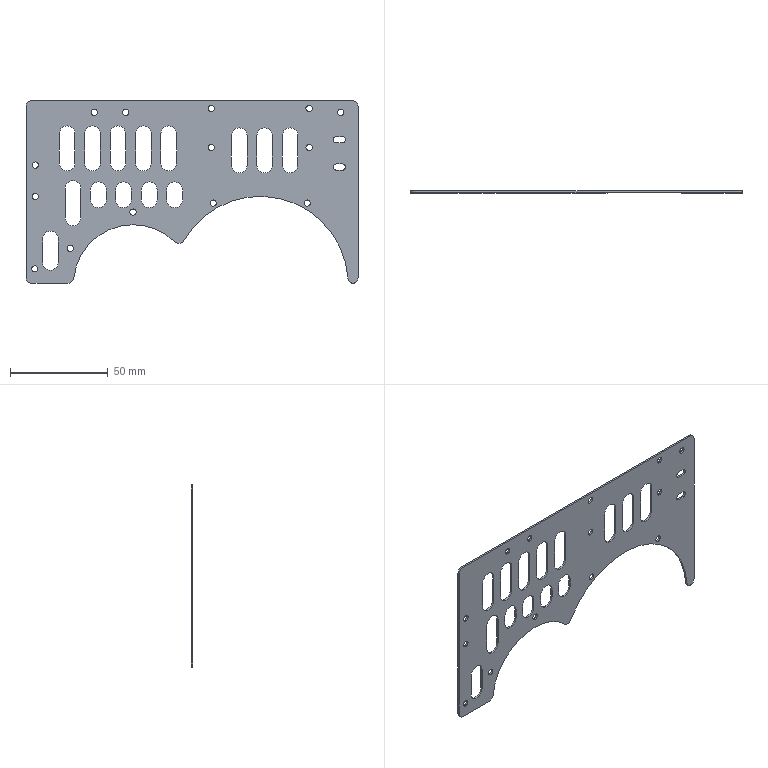Part | SolidWorks | features ICE 12, Fillet 3, Extrusion 1 | 1 solid | 125 faces | box 169.72 x 1 x 93.5 mm | volume 9219 mm3 | cylinder 87 | plane 38 | commonest cylinder face diameters 3.2 x32 8 x30 8.117 x12 6 x8 4 x2 61 x2